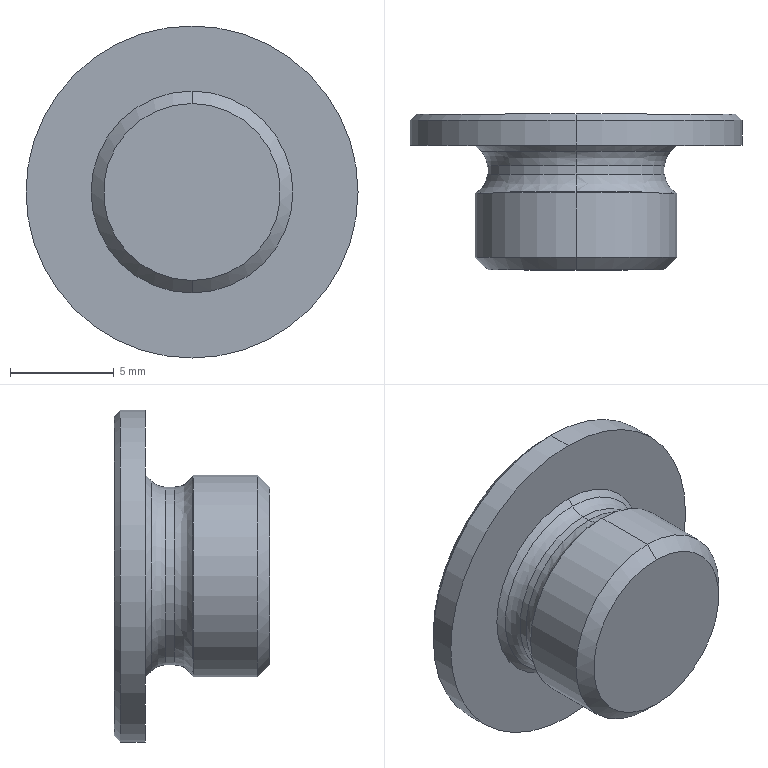Part | STEP file | DGC-25 screw | 1 solid | 30 faces | box 16 x 7.5 x 16 mm | volume 612.752 mm3 | cone 10 | plane 10 | cylinder 6 | spline 4 | commonest cylinder face diameters 8.566 x2 9.728 x2 16 x2